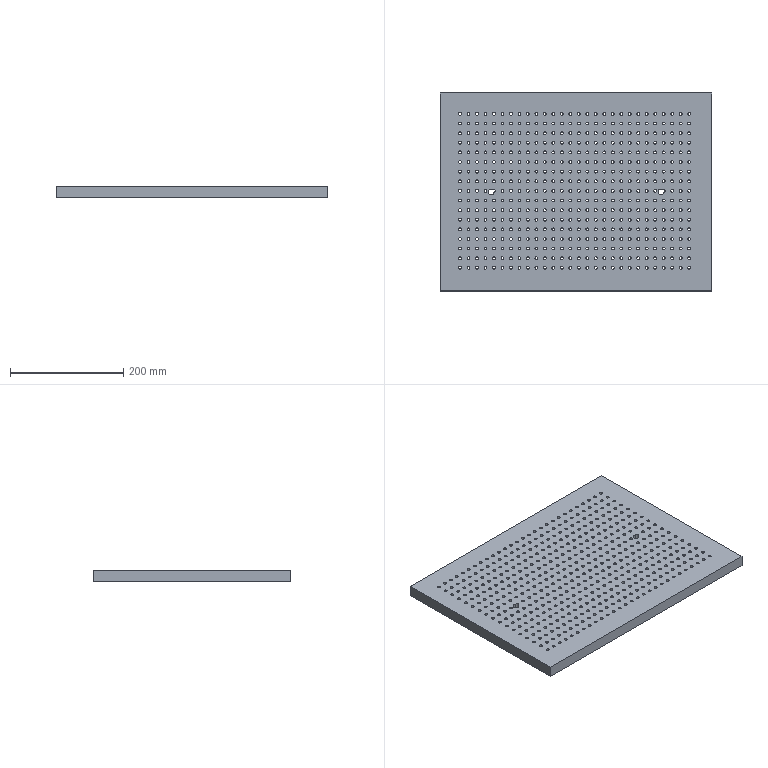Part | STEP file | FCT press block | 1 solid | 958 faces | box 480 x 350 x 20 mm | volume 3170211 mm3 | cylinder 952 | plane 6 | commonest cylinder face diameters 5 x950 10 x2